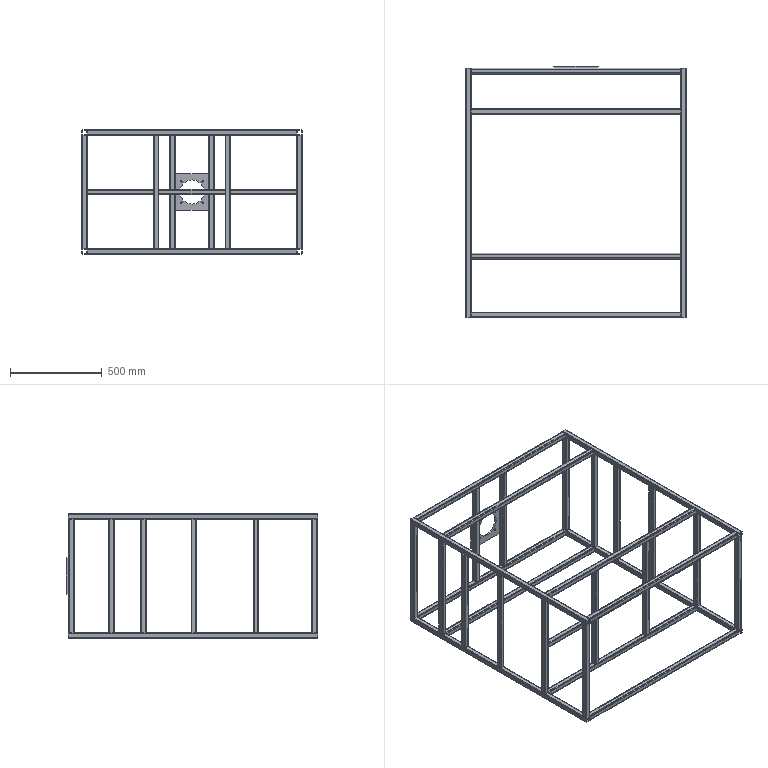Part | SolidWorks | features 3DProfileFeature 1, HoleWzd 1, ICE 1, WeldMemberFeat 1, WeldmentFeature 1 | 32 solids | 574 faces | box 1200 x 1370 x 680 mm | volume 7177358 mm3 | plane 316 | cylinder 258 | commonest cylinder face diameters 5.2 x124 10.4 x124 8.5 x8 132 x2